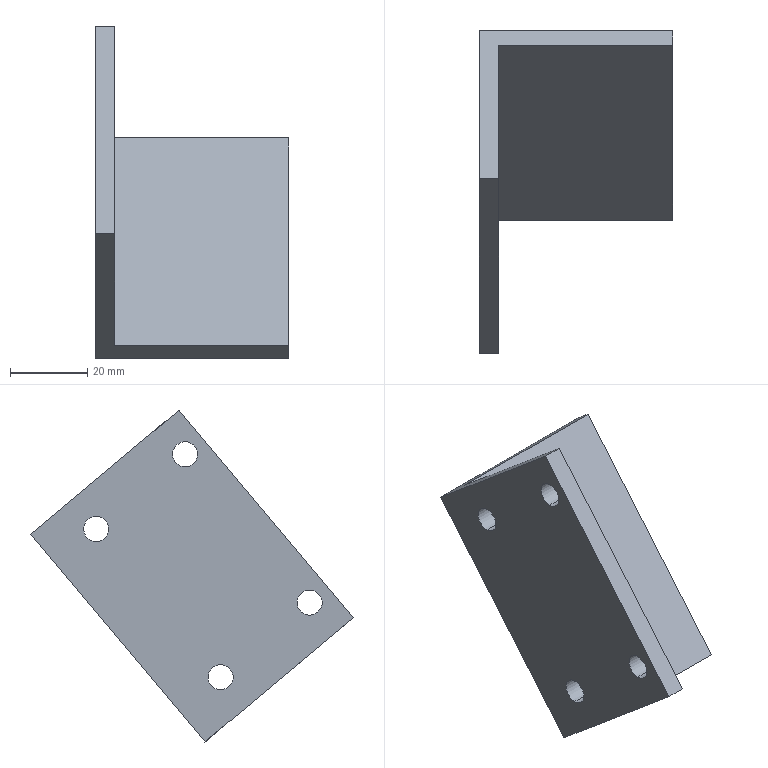Part | SolidWorks | features BaseBody 1 | 1 solid | 16 faces | box 50 x 83.297 x 85.762 mm | volume 32586 mm3 | cylinder 8 | plane 8 | commonest cylinder face diameters 6.5 x8
STEP:
#1=CARTESIAN_POINT('',(190.,93.317,-514.42));
#2=VERTEX_POINT('',#1);
#3=CARTESIAN_POINT('',(190.,93.317,-507.92));
#4=VERTEX_POINT('',#3);
#5=CARTESIAN_POINT('',(190.,93.317,-511.17));
#6=DIRECTION('',(-1.,0.,0.));
#7=DIRECTION('',(0.,0.,-1.));
#8=AXIS2_PLACEMENT_3D('',#5,#6,#7);
#9=CIRCLE('',#8,3.25);
#10=EDGE_CURVE('',#2,#4,#9,.T.);
#11=ORIENTED_EDGE('',*,*,#10,.T.);
#12=CARTESIAN_POINT('',(195.,93.317,-507.92));
#13=VERTEX_POINT('',#12);
#14=CARTESIAN_POINT('',(195.,93.317,-507.92));
#15=DIRECTION('',(1.,0.,0.));
#16=VECTOR('',#15,1000.);
#17=LINE('',#14,#16);
#18=EDGE_CURVE('',#4,#13,#17,.T.);
#19=ORIENTED_EDGE('',*,*,#18,.T.);
#20=CARTESIAN_POINT('',(195.,93.317,-514.42));
#21=VERTEX_POINT('',#20);
#22=CARTESIAN_POINT('',(195.,93.317,-511.17));
#23=DIRECTION('',(1.,0.,0.));
#24=DIRECTION('',(0.,0.,-1.));
#25=AXIS2_PLACEMENT_3D('',#22,#23,#24);
#26=CIRCLE('',#25,3.25);
#27=EDGE_CURVE('',#13,#21,#26,.T.);
#28=ORIENTED_EDGE('',*,*,#27,.T.);
#29=CARTESIAN_POINT('',(195.,93.317,-514.42));
#30=DIRECTION('',(1.,0.,0.));
#31=VECTOR('',#30,1000.);
#32=LINE('',#29,#31);
#33=EDGE_CURVE('',#2,#21,#32,.T.);
#34=ORIENTED_EDGE('',*,*,#33,.F.);
#35=EDGE_LOOP('',(#11,#19,#28,#34));
#36=FACE_OUTER_BOUND('',#35,.T.);
#37=CARTESIAN_POINT('',(195.,93.317,-511.17));
#38=DIRECTION('',(1.,0.,0.));
#39=DIRECTION('',(0.,0.,-1.));
#40=AXIS2_PLACEMENT_3D('',#37,#38,#39);
#41=CYLINDRICAL_SURFACE('',#40,3.25);
#42=ADVANCED_FACE('',(#36),#41,.F.);
#43=CARTESIAN_POINT('',(190.,70.328,-495.146));
#44=VERTEX_POINT('',#43);
#45=CARTESIAN_POINT('',(190.,70.328,-488.646));
#46=VERTEX_POINT('',#45);
#47=CARTESIAN_POINT('',(190.,70.328,-491.896));
#48=DIRECTION('',(-1.,0.,0.));
#49=DIRECTION('',(0.,0.,-1.));
#50=AXIS2_PLACEMENT_3D('',#47,#48,#49);
#51=CIRCLE('',#50,3.25);
#52=EDGE_CURVE('',#44,#46,#51,.T.);
#53=ORIENTED_EDGE('',*,*,#52,.T.);
#54=CARTESIAN_POINT('',(195.,70.328,-488.646));
#55=VERTEX_POINT('',#54);
#56=CARTESIAN_POINT('',(195.,70.328,-488.646));
#57=DIRECTION('',(1.,0.,0.));
#58=VECTOR('',#57,1000.);
#59=LINE('',#56,#58);
#60=EDGE_CURVE('',#46,#55,#59,.T.);
#61=ORIENTED_EDGE('',*,*,#60,.T.);
#62=CARTESIAN_POINT('',(195.,70.328,-495.146));
#63=VERTEX_POINT('',#62);
#64=CARTESIAN_POINT('',(195.,70.328,-491.896));
#65=DIRECTION('',(1.,0.,0.));
#66=DIRECTION('',(0.,0.,-1.));
#67=AXIS2_PLACEMENT_3D('',#64,#65,#66);
#68=CIRCLE('',#67,3.25);
#69=EDGE_CURVE('',#55,#63,#68,.T.);
#70=ORIENTED_EDGE('',*,*,#69,.T.);
#71=CARTESIAN_POINT('',(195.,70.328,-495.146));
#72=DIRECTION('',(1.,0.,0.));
#73=VECTOR('',#72,1000.);
#74=LINE('',#71,#73);
#75=EDGE_CURVE('',#44,#63,#74,.T.);
#76=ORIENTED_EDGE('',*,*,#75,.F.);
#77=EDGE_LOOP('',(#53,#61,#70,#76));
#78=FACE_OUTER_BOUND('',#77,.T.);
#79=CARTESIAN_POINT('',(195.,70.328,-491.896));
#80=DIRECTION('',(1.,0.,0.));
#81=DIRECTION('',(0.,0.,-1.));
#82=AXIS2_PLACEMENT_3D('',#79,#80,#81);
#83=CYLINDRICAL_SURFACE('',#82,3.25);
#84=ADVANCED_FACE('',(#78),#83,.F.);
#85=CARTESIAN_POINT('',(190.,102.467,-456.845));
#86=VERTEX_POINT('',#85);
#87=CARTESIAN_POINT('',(190.,102.467,-450.345));
#88=VERTEX_POINT('',#87);
#89=CARTESIAN_POINT('',(190.,102.467,-453.595));
#90=DIRECTION('',(-1.,0.,0.));
#91=DIRECTION('',(0.,0.,-1.));
#92=AXIS2_PLACEMENT_3D('',#89,#90,#91);
#93=CIRCLE('',#92,3.25);
#94=EDGE_CURVE('',#86,#88,#93,.T.);
#95=ORIENTED_EDGE('',*,*,#94,.T.);
#96=CARTESIAN_POINT('',(195.,102.467,-450.345));
#97=VERTEX_POINT('',#96);
#98=CARTESIAN_POINT('',(195.,102.467,-450.345));
#99=DIRECTION('',(1.,0.,0.));
#100=VECTOR('',#99,1000.);
#101=LINE('',#98,#100);
#102=EDGE_CURVE('',#88,#97,#101,.T.);
#103=ORIENTED_EDGE('',*,*,#102,.T.);
#104=CARTESIAN_POINT('',(195.,102.467,-456.845));
#105=VERTEX_POINT('',#104);
#106=CARTESIAN_POINT('',(195.,102.467,-453.595));
#107=DIRECTION('',(1.,0.,0.));
#108=DIRECTION('',(0.,0.,-1.));
#109=AXIS2_PLACEMENT_3D('',#106,#107,#108);
#110=CIRCLE('',#109,3.25);
#111=EDGE_CURVE('',#97,#105,#110,.T.);
#112=ORIENTED_EDGE('',*,*,#111,.T.);
#113=CARTESIAN_POINT('',(195.,102.467,-456.845));
#114=DIRECTION('',(1.,0.,0.));
#115=VECTOR('',#114,1000.);
#116=LINE('',#113,#115);
#117=EDGE_CURVE('',#86,#105,#116,.T.);
#118=ORIENTED_EDGE('',*,*,#117,.F.);
#119=EDGE_LOOP('',(#95,#103,#112,#118));
#120=FACE_OUTER_BOUND('',#119,.T.);
#121=CARTESIAN_POINT('',(195.,102.467,-453.595));
#122=DIRECTION('',(1.,0.,0.));
#123=DIRECTION('',(0.,0.,-1.));
#124=AXIS2_PLACEMENT_3D('',#121,#122,#123);
#125=CYLINDRICAL_SURFACE('',#124,3.25);
#126=ADVANCED_FACE('',(#120),#125,.F.);
#127=CARTESIAN_POINT('',(190.,125.448,-476.128));
#128=VERTEX_POINT('',#127);
#129=CARTESIAN_POINT('',(190.,125.448,-469.628));
#130=VERTEX_POINT('',#129);
#131=CARTESIAN_POINT('',(190.,125.448,-472.878));
#132=DIRECTION('',(-1.,0.,0.));
#133=DIRECTION('',(0.,0.,-1.));
#134=AXIS2_PLACEMENT_3D('',#131,#132,#133);
#135=CIRCLE('',#134,3.25);
#136=EDGE_CURVE('',#128,#130,#135,.T.);
#137=ORIENTED_EDGE('',*,*,#136,.T.);
#138=CARTESIAN_POINT('',(195.,125.448,-469.628));
#139=VERTEX_POINT('',#138);
#140=CARTESIAN_POINT('',(185.,125.448,-469.628));
#141=DIRECTION('',(1.,0.,0.));
#142=VECTOR('',#141,1000.);
#143=LINE('',#140,#142);
#144=EDGE_CURVE('',#130,#139,#143,.T.);
#145=ORIENTED_EDGE('',*,*,#144,.T.);
#146=CARTESIAN_POINT('',(195.,125.448,-476.128));
#147=VERTEX_POINT('',#146);
#148=CARTESIAN_POINT('',(195.,125.448,-472.878));
#149=DIRECTION('',(1.,0.,0.));
#150=DIRECTION('',(0.,0.,-1.));
#151=AXIS2_PLACEMENT_3D('',#148,#149,#150);
#152=CIRCLE('',#151,3.25);
#153=EDGE_CURVE('',#139,#147,#152,.T.);
#154=ORIENTED_EDGE('',*,*,#153,.T.);
#155=CARTESIAN_POINT('',(185.,125.448,-476.128));
#156=DIRECTION('',(1.,0.,0.));
#157=VECTOR('',#156,1000.);
#158=LINE('',#155,#157);
#159=EDGE_CURVE('',#128,#147,#158,.T.);
#160=ORIENTED_EDGE('',*,*,#159,.F.);
#161=EDGE_LOOP('',(#137,#145,#154,#160));
#162=FACE_OUTER_BOUND('',#161,.T.);
#163=CARTESIAN_POINT('',(185.,125.448,-472.878));
#164=DIRECTION('',(1.,0.,0.));
#165=DIRECTION('',(0.,0.,-1.));
#166=AXIS2_PLACEMENT_3D('',#163,#164,#165);
#167=CYLINDRICAL_SURFACE('',#166,3.25);
#168=ADVANCED_FACE('',(#162),#167,.F.);
#169=CARTESIAN_POINT('',(240.,97.339,-527.905));
#170=VERTEX_POINT('',#169);
#171=CARTESIAN_POINT('',(240.,142.334,-474.282));
#172=VERTEX_POINT('',#171);
#173=CARTESIAN_POINT('',(240.,97.339,-527.905));
#174=DIRECTION('',(0.,0.6428,0.766));
#175=VECTOR('',#174,1000.);
#176=LINE('',#173,#175);
#177=EDGE_CURVE('',#170,#172,#176,.T.);
#178=ORIENTED_EDGE('',*,*,#177,.F.);
#179=CARTESIAN_POINT('',(190.,97.339,-527.905));
#180=VERTEX_POINT('',#179);
#181=CARTESIAN_POINT('',(240.,97.339,-527.905));
#182=DIRECTION('',(1.,0.,0.));
#183=VECTOR('',#182,1000.);
#184=LINE('',#181,#183);
#185=EDGE_CURVE('',#180,#170,#184,.T.);
#186=ORIENTED_EDGE('',*,*,#185,.F.);
#187=CARTESIAN_POINT('',(190.,142.334,-474.282));
#188=VERTEX_POINT('',#187);
#189=CARTESIAN_POINT('',(190.,97.339,-527.905));
#190=DIRECTION('',(0.,-0.6428,-0.766));
#191=VECTOR('',#190,1000.);
#192=LINE('',#189,#191);
#193=EDGE_CURVE('',#188,#180,#192,.T.);
#194=ORIENTED_EDGE('',*,*,#193,.F.);
#195=CARTESIAN_POINT('',(240.,142.334,-474.282));
#196=DIRECTION('',(-1.,0.,0.));
#197=VECTOR('',#196,1000.);
#198=LINE('',#195,#197);
#199=EDGE_CURVE('',#172,#188,#198,.T.);
#200=ORIENTED_EDGE('',*,*,#199,.F.);
#201=EDGE_LOOP('',(#178,#186,#194,#200));
#202=FACE_OUTER_BOUND('',#201,.T.);
#203=CARTESIAN_POINT('',(240.,97.339,-527.905));
#204=DIRECTION('',(0.,-0.766,0.6428));
#205=DIRECTION('',(0.,-0.6428,-0.766));
#206=AXIS2_PLACEMENT_3D('',#203,#204,#205);
#207=PLANE('',#206);
#208=ADVANCED_FACE('',(#202),#207,.F.);
#209=ORIENTED_EDGE('',*,*,#199,.T.);
#210=CARTESIAN_POINT('',(190.,104.032,-442.142));
#211=VERTEX_POINT('',#210);
#212=CARTESIAN_POINT('',(190.,142.334,-474.282));
#213=DIRECTION('',(0.,0.766,-0.6428));
#214=VECTOR('',#213,1000.);
#215=LINE('',#212,#214);
#216=EDGE_CURVE('',#211,#188,#215,.T.);
#217=ORIENTED_EDGE('',*,*,#216,.F.);
#218=CARTESIAN_POINT('',(195.,104.032,-442.142));
#219=VERTEX_POINT('',#218);
#220=CARTESIAN_POINT('',(190.,104.032,-442.142));
#221=DIRECTION('',(-1.,0.,0.));
#222=VECTOR('',#221,1000.);
#223=LINE('',#220,#222);
#224=EDGE_CURVE('',#219,#211,#223,.T.);
#225=ORIENTED_EDGE('',*,*,#224,.F.);
#226=CARTESIAN_POINT('',(195.,138.504,-471.068));
#227=VERTEX_POINT('',#226);
#228=CARTESIAN_POINT('',(195.,142.334,-474.282));
#229=DIRECTION('',(0.,-0.766,0.6428));
#230=VECTOR('',#229,1000.);
#231=LINE('',#228,#230);
#232=EDGE_CURVE('',#227,#219,#231,.T.);
#233=ORIENTED_EDGE('',*,*,#232,.F.);
#234=CARTESIAN_POINT('',(240.,138.504,-471.068));
#235=VERTEX_POINT('',#234);
#236=CARTESIAN_POINT('',(190.,138.504,-471.068));
#237=DIRECTION('',(-1.,0.,0.));
#238=VECTOR('',#237,1000.);
#239=LINE('',#236,#238);
#240=EDGE_CURVE('',#235,#227,#239,.T.);
#241=ORIENTED_EDGE('',*,*,#240,.F.);
#242=CARTESIAN_POINT('',(240.,142.334,-474.282));
#243=DIRECTION('',(0.,-0.766,0.6428));
#244=VECTOR('',#243,1000.);
#245=LINE('',#242,#244);
#246=EDGE_CURVE('',#172,#235,#245,.T.);
#247=ORIENTED_EDGE('',*,*,#246,.F.);
#248=EDGE_LOOP('',(#209,#217,#225,#233,#241,#247));
#249=FACE_OUTER_BOUND('',#248,.T.);
#250=CARTESIAN_POINT('',(190.,142.334,-474.282));
#251=DIRECTION('',(0.,-0.6428,-0.766));
#252=DIRECTION('',(0.,0.766,-0.6428));
#253=AXIS2_PLACEMENT_3D('',#250,#251,#252);
#254=PLANE('',#253);
#255=ADVANCED_FACE('',(#249),#254,.F.);
#256=CARTESIAN_POINT('',(240.,93.509,-524.691));
#257=VERTEX_POINT('',#256);
#258=CARTESIAN_POINT('',(240.,93.509,-524.691));
#259=DIRECTION('',(0.,0.6428,0.766));
#260=VECTOR('',#259,1000.);
#261=LINE('',#258,#260);
#262=EDGE_CURVE('',#257,#235,#261,.T.);
#263=ORIENTED_EDGE('',*,*,#262,.F.);
#264=CARTESIAN_POINT('',(240.,97.339,-527.905));
#265=DIRECTION('',(0.,-0.766,0.6428));
#266=VECTOR('',#265,1000.);
#267=LINE('',#264,#266);
#268=EDGE_CURVE('',#170,#257,#267,.T.);
#269=ORIENTED_EDGE('',*,*,#268,.F.);
#270=ORIENTED_EDGE('',*,*,#177,.T.);
#271=ORIENTED_EDGE('',*,*,#246,.T.);
#272=EDGE_LOOP('',(#263,#269,#270,#271));
#273=FACE_OUTER_BOUND('',#272,.T.);
#274=CARTESIAN_POINT('',(240.,97.339,-527.905));
#275=DIRECTION('',(-1.,0.,0.));
#276=DIRECTION('',(0.,0.,1.));
#277=AXIS2_PLACEMENT_3D('',#274,#275,#276);
#278=PLANE('',#277);
#279=ADVANCED_FACE('',(#273),#278,.F.);
#280=CARTESIAN_POINT('',(190.,59.037,-495.766));
#281=VERTEX_POINT('',#280);
#282=CARTESIAN_POINT('',(190.,97.339,-527.905));
#283=DIRECTION('',(0.,0.766,-0.6428));
#284=VECTOR('',#283,1000.);
#285=LINE('',#282,#284);
#286=EDGE_CURVE('',#281,#180,#285,.T.);
#287=ORIENTED_EDGE('',*,*,#286,.T.);
#288=ORIENTED_EDGE('',*,*,#185,.T.);
#289=ORIENTED_EDGE('',*,*,#268,.T.);
#290=CARTESIAN_POINT('',(195.,93.509,-524.691));
#291=VERTEX_POINT('',#290);
#292=CARTESIAN_POINT('',(190.,93.509,-524.691));
#293=DIRECTION('',(-1.,0.,0.));
#294=VECTOR('',#293,1000.);
#295=LINE('',#292,#294);
#296=EDGE_CURVE('',#257,#291,#295,.T.);
#297=ORIENTED_EDGE('',*,*,#296,.T.);
#298=CARTESIAN_POINT('',(195.,59.037,-495.766));
#299=VERTEX_POINT('',#298);
#300=CARTESIAN_POINT('',(195.,97.339,-527.905));
#301=DIRECTION('',(0.,-0.766,0.6428));
#302=VECTOR('',#301,1000.);
#303=LINE('',#300,#302);
#304=EDGE_CURVE('',#291,#299,#303,.T.);
#305=ORIENTED_EDGE('',*,*,#304,.T.);
#306=CARTESIAN_POINT('',(190.,59.037,-495.766));
#307=DIRECTION('',(-1.,0.,0.));
#308=VECTOR('',#307,1000.);
#309=LINE('',#306,#308);
#310=EDGE_CURVE('',#299,#281,#309,.T.);
#311=ORIENTED_EDGE('',*,*,#310,.T.);
#312=EDGE_LOOP('',(#287,#288,#289,#297,#305,#311));
#313=FACE_OUTER_BOUND('',#312,.T.);
#314=CARTESIAN_POINT('',(190.,97.339,-527.905));
#315=DIRECTION('',(0.,-0.6428,-0.766));
#316=DIRECTION('',(0.,0.766,-0.6428));
#317=AXIS2_PLACEMENT_3D('',#314,#315,#316);
#318=PLANE('',#317);
#319=ADVANCED_FACE('',(#313),#318,.T.);
#320=ORIENTED_EDGE('',*,*,#193,.T.);
#321=ORIENTED_EDGE('',*,*,#286,.F.);
#322=CARTESIAN_POINT('',(190.,104.032,-442.142));
#323=DIRECTION('',(0.,-0.6428,-0.766));
#324=VECTOR('',#323,1000.);
#325=LINE('',#322,#324);
#326=EDGE_CURVE('',#211,#281,#325,.T.);
#327=ORIENTED_EDGE('',*,*,#326,.F.);
#328=ORIENTED_EDGE('',*,*,#216,.T.);
#329=EDGE_LOOP('',(#320,#321,#327,#328));
#330=FACE_OUTER_BOUND('',#329,.T.);
#331=ORIENTED_EDGE('',*,*,#10,.F.);
#332=CARTESIAN_POINT('',(190.,93.317,-511.17));
#333=DIRECTION('',(-1.,0.,0.));
#334=DIRECTION('',(0.,0.,-1.));
#335=AXIS2_PLACEMENT_3D('',#332,#333,#334);
#336=CIRCLE('',#335,3.25);
#337=EDGE_CURVE('',#4,#2,#336,.T.);
#338=ORIENTED_EDGE('',*,*,#337,.F.);
#339=EDGE_LOOP('',(#331,#338));
#340=FACE_BOUND('',#339,.T.);
#341=ORIENTED_EDGE('',*,*,#52,.F.);
#342=CARTESIAN_POINT('',(190.,70.328,-491.896));
#343=DIRECTION('',(-1.,0.,0.));
#344=DIRECTION('',(0.,0.,-1.));
#345=AXIS2_PLACEMENT_3D('',#342,#343,#344);
#346=CIRCLE('',#345,3.25);
#347=EDGE_CURVE('',#46,#44,#346,.T.);
#348=ORIENTED_EDGE('',*,*,#347,.F.);
#349=EDGE_LOOP('',(#341,#348));
#350=FACE_BOUND('',#349,.T.);
#351=ORIENTED_EDGE('',*,*,#94,.F.);
#352=CARTESIAN_POINT('',(190.,102.467,-453.595));
#353=DIRECTION('',(-1.,0.,0.));
#354=DIRECTION('',(0.,0.,-1.));
#355=AXIS2_PLACEMENT_3D('',#352,#353,#354);
#356=CIRCLE('',#355,3.25);
#357=EDGE_CURVE('',#88,#86,#356,.T.);
#358=ORIENTED_EDGE('',*,*,#357,.F.);
#359=EDGE_LOOP('',(#351,#358));
#360=FACE_BOUND('',#359,.T.);
#361=ORIENTED_EDGE('',*,*,#136,.F.);
#362=CARTESIAN_POINT('',(190.,125.448,-472.878));
#363=DIRECTION('',(-1.,0.,0.));
#364=DIRECTION('',(0.,0.,-1.));
#365=AXIS2_PLACEMENT_3D('',#362,#363,#364);
#366=CIRCLE('',#365,3.25);
#367=EDGE_CURVE('',#130,#128,#366,.T.);
#368=ORIENTED_EDGE('',*,*,#367,.F.);
#369=EDGE_LOOP('',(#361,#368));
#370=FACE_BOUND('',#369,.T.);
#371=CARTESIAN_POINT('',(190.,97.339,-527.905));
#372=DIRECTION('',(1.,0.,0.));
#373=DIRECTION('',(0.,0.,-1.));
#374=AXIS2_PLACEMENT_3D('',#371,#372,#373);
#375=PLANE('',#374);
#376=ADVANCED_FACE('',(#330,#340,#350,#360,#370),#375,.F.);
#377=ORIENTED_EDGE('',*,*,#326,.T.);
#378=ORIENTED_EDGE('',*,*,#310,.F.);
#379=CARTESIAN_POINT('',(195.,59.037,-495.766));
#380=DIRECTION('',(0.,-0.6428,-0.766));
#381=VECTOR('',#380,1000.);
#382=LINE('',#379,#381);
#383=EDGE_CURVE('',#219,#299,#382,.T.);
#384=ORIENTED_EDGE('',*,*,#383,.F.);
#385=ORIENTED_EDGE('',*,*,#224,.T.);
#386=EDGE_LOOP('',(#377,#378,#384,#385));
#387=FACE_OUTER_BOUND('',#386,.T.);
#388=CARTESIAN_POINT('',(195.,59.037,-495.766));
#389=DIRECTION('',(0.,0.766,-0.6428));
#390=DIRECTION('',(0.,0.6428,0.766));
#391=AXIS2_PLACEMENT_3D('',#388,#389,#390);
#392=PLANE('',#391);
#393=ADVANCED_FACE('',(#387),#392,.F.);
#394=ORIENTED_EDGE('',*,*,#383,.T.);
#395=ORIENTED_EDGE('',*,*,#304,.F.);
#396=CARTESIAN_POINT('',(195.,138.504,-471.068));
#397=DIRECTION('',(0.,-0.6428,-0.766));
#398=VECTOR('',#397,1000.);
#399=LINE('',#396,#398);
#400=EDGE_CURVE('',#227,#291,#399,.T.);
#401=ORIENTED_EDGE('',*,*,#400,.F.);
#402=ORIENTED_EDGE('',*,*,#232,.T.);
#403=EDGE_LOOP('',(#394,#395,#401,#402));
#404=FACE_OUTER_BOUND('',#403,.T.);
#405=CARTESIAN_POINT('',(195.,93.317,-511.17));
#406=DIRECTION('',(1.,0.,0.));
#407=DIRECTION('',(0.,0.,-1.));
#408=AXIS2_PLACEMENT_3D('',#405,#406,#407);
#409=CIRCLE('',#408,3.25);
#410=EDGE_CURVE('',#21,#13,#409,.T.);
#411=ORIENTED_EDGE('',*,*,#410,.F.);
#412=ORIENTED_EDGE('',*,*,#27,.F.);
#413=EDGE_LOOP('',(#411,#412));
#414=FACE_BOUND('',#413,.T.);
#415=CARTESIAN_POINT('',(195.,70.328,-491.896));
#416=DIRECTION('',(1.,0.,0.));
#417=DIRECTION('',(0.,0.,-1.));
#418=AXIS2_PLACEMENT_3D('',#415,#416,#417);
#419=CIRCLE('',#418,3.25);
#420=EDGE_CURVE('',#63,#55,#419,.T.);
#421=ORIENTED_EDGE('',*,*,#420,.F.);
#422=ORIENTED_EDGE('',*,*,#69,.F.);
#423=EDGE_LOOP('',(#421,#422));
#424=FACE_BOUND('',#423,.T.);
#425=CARTESIAN_POINT('',(195.,102.467,-453.595));
#426=DIRECTION('',(1.,0.,0.));
#427=DIRECTION('',(0.,0.,-1.));
#428=AXIS2_PLACEMENT_3D('',#425,#426,#427);
#429=CIRCLE('',#428,3.25);
#430=EDGE_CURVE('',#105,#97,#429,.T.);
#431=ORIENTED_EDGE('',*,*,#430,.F.);
#432=ORIENTED_EDGE('',*,*,#111,.F.);
#433=EDGE_LOOP('',(#431,#432));
#434=FACE_BOUND('',#433,.T.);
#435=CARTESIAN_POINT('',(195.,125.448,-472.878));
#436=DIRECTION('',(1.,0.,0.));
#437=DIRECTION('',(0.,0.,-1.));
#438=AXIS2_PLACEMENT_3D('',#435,#436,#437);
#439=CIRCLE('',#438,3.25);
#440=EDGE_CURVE('',#147,#139,#439,.T.);
#441=ORIENTED_EDGE('',*,*,#440,.F.);
#442=ORIENTED_EDGE('',*,*,#153,.F.);
#443=EDGE_LOOP('',(#441,#442));
#444=FACE_BOUND('',#443,.T.);
#445=CARTESIAN_POINT('',(195.,93.509,-524.691));
#446=DIRECTION('',(-1.,0.,0.));
#447=DIRECTION('',(0.,0.,1.));
#448=AXIS2_PLACEMENT_3D('',#445,#446,#447);
#449=PLANE('',#448);
#450=ADVANCED_FACE('',(#404,#414,#424,#434,#444),#449,.F.);
#451=ORIENTED_EDGE('',*,*,#400,.T.);
#452=ORIENTED_EDGE('',*,*,#296,.F.);
#453=ORIENTED_EDGE('',*,*,#262,.T.);
#454=ORIENTED_EDGE('',*,*,#240,.T.);
#455=EDGE_LOOP('',(#451,#452,#453,#454));
#456=FACE_OUTER_BOUND('',#455,.T.);
#457=CARTESIAN_POINT('',(240.,93.509,-524.691));
#458=DIRECTION('',(0.,0.766,-0.6428));
#459=DIRECTION('',(0.,0.6428,0.766));
#460=AXIS2_PLACEMENT_3D('',#457,#458,#459);
#461=PLANE('',#460);
#462=ADVANCED_FACE('',(#456),#461,.F.);
#463=ORIENTED_EDGE('',*,*,#18,.F.);
#464=ORIENTED_EDGE('',*,*,#337,.T.);
#465=ORIENTED_EDGE('',*,*,#33,.T.);
#466=ORIENTED_EDGE('',*,*,#410,.T.);
#467=EDGE_LOOP('',(#463,#464,#465,#466));
#468=FACE_OUTER_BOUND('',#467,.T.);
#469=CARTESIAN_POINT('',(195.,93.317,-511.17));
#470=DIRECTION('',(1.,0.,0.));
#471=DIRECTION('',(0.,0.,-1.));
#472=AXIS2_PLACEMENT_3D('',#469,#470,#471);
#473=CYLINDRICAL_SURFACE('',#472,3.25);
#474=ADVANCED_FACE('',(#468),#473,.F.);
#475=ORIENTED_EDGE('',*,*,#60,.F.);
#476=ORIENTED_EDGE('',*,*,#347,.T.);
#477=ORIENTED_EDGE('',*,*,#75,.T.);
#478=ORIENTED_EDGE('',*,*,#420,.T.);
#479=EDGE_LOOP('',(#475,#476,#477,#478));
#480=FACE_OUTER_BOUND('',#479,.T.);
#481=CARTESIAN_POINT('',(195.,70.328,-491.896));
#482=DIRECTION('',(1.,0.,0.));
#483=DIRECTION('',(0.,0.,-1.));
#484=AXIS2_PLACEMENT_3D('',#481,#482,#483);
#485=CYLINDRICAL_SURFACE('',#484,3.25);
#486=ADVANCED_FACE('',(#480),#485,.F.);
#487=ORIENTED_EDGE('',*,*,#102,.F.);
#488=ORIENTED_EDGE('',*,*,#357,.T.);
#489=ORIENTED_EDGE('',*,*,#117,.T.);
#490=ORIENTED_EDGE('',*,*,#430,.T.);
#491=EDGE_LOOP('',(#487,#488,#489,#490));
#492=FACE_OUTER_BOUND('',#491,.T.);
#493=CARTESIAN_POINT('',(195.,102.467,-453.595));
#494=DIRECTION('',(1.,0.,0.));
#495=DIRECTION('',(0.,0.,-1.));
#496=AXIS2_PLACEMENT_3D('',#493,#494,#495);
#497=CYLINDRICAL_SURFACE('',#496,3.25);
#498=ADVANCED_FACE('',(#492),#497,.F.);
#499=ORIENTED_EDGE('',*,*,#144,.F.);
#500=ORIENTED_EDGE('',*,*,#367,.T.);
#501=ORIENTED_EDGE('',*,*,#159,.T.);
#502=ORIENTED_EDGE('',*,*,#440,.T.);
#503=EDGE_LOOP('',(#499,#500,#501,#502));
#504=FACE_OUTER_BOUND('',#503,.T.);
#505=CARTESIAN_POINT('',(185.,125.448,-472.878));
#506=DIRECTION('',(1.,0.,0.));
#507=DIRECTION('',(0.,0.,-1.));
#508=AXIS2_PLACEMENT_3D('',#505,#506,#507);
#509=CYLINDRICAL_SURFACE('',#508,3.25);
#510=ADVANCED_FACE('',(#504),#509,.F.);
#511=CLOSED_SHELL('',(#42,#84,#126,#168,#208,#255,#279,#319,#376,#393,#450,#462,#474,#486,#498,#510));
#512=MANIFOLD_SOLID_BREP('',#511);
#513=CARTESIAN_POINT('',(0.,0.,0.));
#514=DIRECTION('',(0.,0.,1.));
#515=DIRECTION('',(1.,0.,0.));
#516=AXIS2_PLACEMENT_3D('',#513,#514,#515);
#517=(LENGTH_UNIT()NAMED_UNIT(*)SI_UNIT(.MILLI.,.METRE.));
#518=UNCERTAINTY_MEASURE_WITH_UNIT(LENGTH_MEASURE(0.00001),#517,'','');
#519=(NAMED_UNIT(*)PLANE_ANGLE_UNIT()SI_UNIT($,.RADIAN.));
#520=(NAMED_UNIT(*)SI_UNIT($,.STERADIAN.)SOLID_ANGLE_UNIT());
#521=(GEOMETRIC_REPRESENTATION_CONTEXT(3)GLOBAL_UNCERTAINTY_ASSIGNED_CONTEXT((#518))GLOBAL_UNIT_ASSIGNED_CONTEXT((#517,#519,#520))REPRESENTATION_CONTEXT('',''));
#522=ADVANCED_BREP_SHAPE_REPRESENTATION('',(#512,#516),#521);